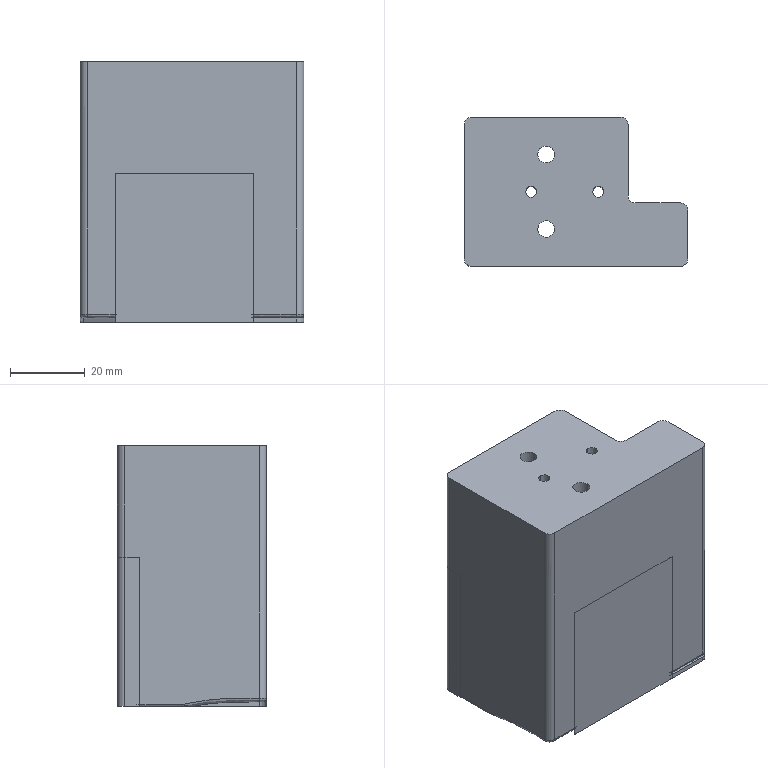NC program | NX | posted with a generic post | part box 60.004 x 40.015 x 70 mm
Lines 1 to 1318 of 2490:
N10 G17 G21 G94 G90
(FLOOR_WALL , TOOL : D63)
N12 T01 M6
N14 G54
N16 G17 G0 G90 X-72.5 Y32.997 B0. C0. S6500 M3
N18 G43 Z30. H1
N20 Z3.
N22 G94 G1 Z0. F1250.
N24 X-69.5
N26 X69.5
N28 Y12.597
N30 X-69.5
N32 Y-7.804
N34 X69.5
N36 X72.5
N38 Z3.
N40 G0 Z30.
N42 M5
(CAVITY_MILL , TOOL : D10)
N44 T09 M6
N46 G54
N48 G17 G0 G90 X4.33 Y-40. B0. C0. S9500 M3
N50 G43 Z30. H9
N52 Z0.504
N54 G94 G1 Z-0.996 F1000.
N56 X0.866 Y-34.
N58 G3 X0. Y-33.5 R1.
N60 G1 X-38.002 F3000.
N62 G2 X-38.495 Y-33.007 R0.493
N64 G1 Y-18.972
N66 G2 X-41.3 Y-13.732 R6.329
N68 G1 Y29.736
N70 G2 X-35. Y36.044 R6.328
N72 G1 X-5.019
N74 X35.006
N76 G2 X41.3 Y29.732 R6.327
N78 G1 Y-13.731
N80 G2 X38.495 Y-18.983 R6.306
N82 G1 Y-33.007
N84 G2 X38.002 Y-33.5 R0.493
N86 G1 X0.
N88 Y-27.5
N90 X-32.495
N92 Y-20.044
N94 X32.495
N96 Y-18.844
N98 X-35.
N100 G2 X-40.1 Y-13.732 R5.129
N102 G1 Y29.732
N104 G2 X-35. Y34.844 R5.128
N106 G1 X35.
N108 G2 X40.1 Y29.732 R5.127
N110 G1 Y-13.732
N112 G2 X35. Y-18.844 R5.106
N114 G1 X32.495
N116 Y-20.044
N118 Y-27.5
N120 X0.
N122 G3 X-0.866 Y-28. R1.
N124 G1 Y-40.
N126 Z0.504
N128 G0 X4.33 Z-0.491
N130 G1 Z-1.991 F1000.
N132 X0.866 Y-34.
N134 G3 X0. Y-33.5 R1.
N136 G1 X-38.002 F3000.
N138 G2 X-38.495 Y-33.007 R0.493
N140 G1 Y-19.24
N142 G2 X-41.3 Y-14. R6.299
N144 G1 Y30.
N146 G2 X-35. Y36.299 R6.3
N148 G1 X35.025 Y36.296
N150 X35.263 Y36.291
N152 G2 X41.3 Y30. R6.295
N154 G1 Y-14.
N156 G2 X38.495 Y-19.24 R6.3
N158 G1 Y-33.007
N160 G2 X38.002 Y-33.5 R0.493
N162 G1 X0.
N164 Y-27.5
N166 X-32.495
N168 Y-20.299
N170 X32.495
N172 Y-19.099
N174 X-35.001
N176 G2 X-40.1 Y-14. R5.099
N178 G1 Y30.
N180 G2 X-35. Y35.099 R5.1
N182 G1 X35. Y35.096
N184 X35.214 Y35.092
N186 G2 X40.1 Y30. R5.095
N188 G1 Y-14.
N190 G2 X35.013 Y-19.099 R5.1
N192 G1 X32.495
N194 Y-20.299
N196 Y-27.5
N198 X0.
N200 G3 X-0.866 Y-28. R1.
N202 G1 Y-40.
N204 Z-0.491
N206 G0 X4.33 Z-1.487
N208 G1 Z-2.987 F1000.
N210 X0.866 Y-34.
N212 G3 X0. Y-33.5 R1.
N214 G1 X-38.002 F3000.
N216 G2 X-38.496 Y-33.007 R0.493
N218 G1 Y-19.241
N220 G2 X-41.3 Y-14. R6.3
N222 G1 Y30.
N224 G2 X-35. Y36.3 R6.3
N226 G1 X35.
N228 G2 X41.3 Y30. R6.3
N230 G1 Y-14.
N232 G2 X38.496 Y-19.241 R6.3
N234 G1 Y-33.007
N236 G2 X38.002 Y-33.5 R0.493
N238 G1 X0.
N240 Y-27.5
N242 X-32.496
N244 Y-20.3
N246 X32.496
N248 Y-19.1
N250 X-35.
N252 G2 X-40.1 Y-14. R5.1
N254 G1 Y30.
N256 G2 X-35. Y35.1 R5.1
N258 G1 X35.
N260 G2 X40.1 Y30. R5.1
N262 G1 Y-14.
N264 G2 X35. Y-19.1 R5.1
N266 G1 X32.496
N268 Y-20.3
N270 Y-27.5
N272 X0.
N274 G3 X-0.866 Y-28. R1.
N276 G1 Y-40.
N278 Z-1.487
N280 G0 X4.33 Z-2.483
N282 G1 Z-3.983 F1000.
N284 X0.866 Y-34.
N286 G3 X0. Y-33.5 R1.
N288 G1 X-38.002 F3000.
N290 G2 X-38.496 Y-33.007 R0.493
N292 G1 Y-19.241
N294 G2 X-41.3 Y-14. R6.3
N296 G1 Y30.
N298 G2 X-35. Y36.3 R6.3
N300 G1 X35.
N302 G2 X41.3 Y30. R6.3
N304 G1 Y-14.
N306 G2 X38.496 Y-19.241 R6.3
N308 G1 Y-33.007
N310 G2 X38.002 Y-33.5 R0.493
N312 G1 X0.
N314 Y-27.5
N316 X-32.496
N318 Y-20.3
N320 X32.496
N322 Y-19.1
N324 X-35.
N326 G2 X-40.1 Y-14. R5.1
N328 G1 Y30.
N330 G2 X-35. Y35.1 R5.1
N332 G1 X35.
N334 G2 X40.1 Y30. R5.1
N336 G1 Y-14.
N338 G2 X35. Y-19.1 R5.1
N340 G1 X32.496
N342 Y-20.3
N344 Y-27.5
N346 X0.
N348 G3 X-0.866 Y-28. R1.
N350 G1 Y-40.
N352 Z-2.483
N354 G0 X4.33 Z-3.478
N356 G1 Z-4.978 F1000.
N358 X0.866 Y-34.
N360 G3 X0. Y-33.5 R1.
N362 G1 X-38.002 F3000.
N364 G2 X-38.496 Y-33.007 R0.494
N366 G1 Y-19.241
N368 G2 X-41.3 Y-14. R6.3
N370 G1 Y30.
N372 G2 X-35. Y36.3 R6.3
N374 G1 X35.
N376 G2 X41.3 Y30. R6.3
N378 G1 Y-14.
N380 G2 X38.496 Y-19.241 R6.3
N382 G1 Y-33.007
N384 G2 X38.002 Y-33.5 R0.494
N386 G1 X0.
N388 Y-27.5
N390 X-32.496
N392 Y-20.3
N394 X32.496
N396 Y-19.1
N398 X-35.
N400 G2 X-40.1 Y-14. R5.1
N402 G1 Y30.
N404 G2 X-35. Y35.1 R5.1
N406 G1 X35.
N408 G2 X40.1 Y30. R5.1
N410 G1 Y-14.
N412 G2 X35. Y-19.1 R5.1
N414 G1 X32.496
N416 Y-20.3
N418 Y-27.5
N420 X0.
N422 G3 X-0.866 Y-28. R1.
N424 G1 Y-40.
N426 Z-3.478
N428 G0 X4.33 Z-4.474
N430 G1 Z-5.974 F1000.
N432 X0.866 Y-34.
N434 G3 X0. Y-33.5 R1.
N436 G1 X-38.002 F3000.
N438 G2 X-38.496 Y-33.007 R0.494
N440 G1 Y-19.241
N442 G2 X-41.3 Y-14. R6.3
N444 G1 Y30.
N446 G2 X-35. Y36.3 R6.3
N448 G1 X35.
N450 G2 X41.3 Y30. R6.3
N452 G1 Y-14.
N454 G2 X38.496 Y-19.241 R6.3
N456 G1 Y-33.007
N458 G2 X38.002 Y-33.5 R0.494
N460 G1 X0.
N462 Y-27.5
N464 X-32.496
N466 Y-20.3
N468 X32.496
N470 Y-19.1
N472 X-35.
N474 G2 X-40.1 Y-14. R5.1
N476 G1 Y30.
N478 G2 X-35. Y35.1 R5.1
N480 G1 X35.
N482 G2 X40.1 Y30. R5.1
N484 G1 Y-14.
N486 G2 X35. Y-19.1 R5.1
N488 G1 X32.496
N490 Y-20.3
N492 Y-27.5
N494 X0.
N496 G3 X-0.866 Y-28. R1.
N498 G1 Y-40.
N500 Z-4.474
N502 G0 X4.33 Y-40.001 Z-5.47
N504 G1 Z-6.97 F1000.
N506 X0.866 Y-34.001
N508 G3 X0. Y-33.501 R1.
N510 G1 X-38.002 F3000.
N512 G2 X-38.496 Y-33.007 R0.494
N514 G1 Y-19.241
N516 G2 X-41.3 Y-14. R6.3
N518 G1 Y30.
N520 G2 X-35. Y36.3 R6.3
N522 G1 X35.
N524 G2 X41.3 Y30. R6.3
N526 G1 Y-14.
N528 G2 X38.496 Y-19.241 R6.3
N530 G1 Y-33.007
N532 G2 X38.002 Y-33.501 R0.494
N534 G1 X0.
N536 Y-27.501
N538 X-32.496
N540 Y-20.3
N542 X32.496
N544 Y-19.1
N546 X-35.
N548 G2 X-40.1 Y-14. R5.1
N550 G1 Y30.
N552 G2 X-35. Y35.1 R5.1
N554 G1 X35.
N556 G2 X40.1 Y30. R5.1
N558 G1 Y-14.
N560 G2 X35. Y-19.1 R5.1
N562 G1 X32.496
N564 Y-20.3
N566 Y-27.501
N568 X0.
N570 G3 X-0.866 Y-28.001 R1.
N572 G1 Y-40.001
N574 Z-5.47
N576 G0 X4.33 Z-6.465
N578 G1 Z-7.965 F1000.
N580 X0.866 Y-34.001
N582 G3 X0. Y-33.501 R1.
N584 G1 X-38.002 F3000.
N586 G2 X-38.496 Y-33.007 R0.494
N588 G1 Y-19.241
N590 G2 X-41.3 Y-14. R6.3
N592 G1 Y30.
N594 G2 X-35. Y36.3 R6.3
N596 G1 X35.
N598 G2 X41.3 Y30. R6.3
N600 G1 Y-14.
N602 G2 X38.496 Y-19.241 R6.3
N604 G1 Y-33.007
N606 G2 X38.002 Y-33.501 R0.494
N608 G1 X0.
N610 Y-27.501
N612 X-32.496
N614 Y-20.3
N616 X32.496
N618 Y-19.1
N620 X-35.
N622 G2 X-40.1 Y-14. R5.1
N624 G1 Y30.
N626 G2 X-35. Y35.1 R5.1
N628 G1 X35.
N630 G2 X40.1 Y30. R5.1
N632 G1 Y-14.
N634 G2 X35. Y-19.1 R5.1
N636 G1 X32.496
N638 Y-20.3
N640 Y-27.501
N642 X0.
N644 G3 X-0.866 Y-28.001 R1.
N646 G1 Y-40.001
N648 Z-6.465
N650 G0 X4.33 Z-7.461
N652 G1 Z-8.961 F1000.
N654 X0.866 Y-34.001
N656 G3 X0. Y-33.501 R1.
N658 G1 X-38.002 F3000.
N660 G2 X-38.496 Y-33.007 R0.494
N662 G1 Y-19.241
N664 G2 X-41.3 Y-14. R6.3
N666 G1 Y30.
N668 G2 X-35. Y36.3 R6.3
N670 G1 X35.
N672 G2 X41.3 Y30. R6.3
N674 G1 Y-14.
N676 G2 X38.496 Y-19.241 R6.3
N678 G1 Y-33.007
N680 G2 X38.002 Y-33.501 R0.494
N682 G1 X0.
N684 Y-27.501
N686 X-32.496
N688 Y-20.3
N690 X32.496
N692 Y-19.1
N694 X-35.
N696 G2 X-40.1 Y-14. R5.1
N698 G1 Y30.
N700 G2 X-35. Y35.1 R5.1
N702 G1 X35.
N704 G2 X40.1 Y30. R5.1
N706 G1 Y-14.
N708 G2 X35. Y-19.1 R5.1
N710 G1 X32.496
N712 Y-20.3
N714 Y-27.501
N716 X0.
N718 G3 X-0.866 Y-28.001 R1.
N720 G1 Y-40.001
N722 Z-7.461
N724 G0 X4.33 Z-8.457
N726 G1 Z-9.957 F1000.
N728 X0.866 Y-34.001
N730 G3 X0. Y-33.501 R1.
N732 G1 X-38.002 F3000.
N734 G2 X-38.496 Y-33.007 R0.494
N736 G1 Y-19.241
N738 G2 X-41.3 Y-14. R6.3
N740 G1 Y30.
N742 G2 X-35. Y36.3 R6.3
N744 G1 X35.
N746 G2 X41.3 Y30. R6.3
N748 G1 Y-14.
N750 G2 X38.496 Y-19.241 R6.3
N752 G1 Y-33.007
N754 G2 X38.002 Y-33.501 R0.494
N756 G1 X0.
N758 Y-27.501
N760 X-32.496
N762 Y-20.3
N764 X32.496
N766 Y-19.1
N768 X-35.
N770 G2 X-40.1 Y-14. R5.1
N772 G1 Y30.
N774 G2 X-35. Y35.1 R5.1
N776 G1 X35.
N778 G2 X40.1 Y30. R5.1
N780 G1 Y-14.
N782 G2 X35. Y-19.1 R5.1
N784 G1 X32.496
N786 Y-20.3
N788 Y-27.501
N790 X0.
N792 G3 X-0.866 Y-28.001 R1.
N794 G1 Y-40.001
N796 Z-8.457
N798 G0 X4.33 Z-9.452
N800 G1 Z-10.952 F1000.
N802 X0.866 Y-34.001
N804 G3 X0. Y-33.501 R1.
N806 G1 X-38.002 F3000.
N808 G2 X-38.496 Y-33.006 R0.494
N810 G1 Y-19.241
N812 G2 X-41.3 Y-14. R6.3
N814 G1 Y30.
N816 G2 X-35. Y36.3 R6.3
N818 G1 X35.
N820 G2 X41.3 Y30. R6.3
N822 G1 Y-14.
N824 G2 X38.496 Y-19.241 R6.3
N826 G1 Y-33.006
N828 G2 X38.002 Y-33.501 R0.494
N830 G1 X0.
N832 Y-27.501
N834 X-32.496
N836 Y-20.3
N838 X32.496
N840 Y-19.1
N842 X-35.
N844 G2 X-40.1 Y-14. R5.1
N846 G1 Y30.
N848 G2 X-35. Y35.1 R5.1
N850 G1 X35.
N852 G2 X40.1 Y30. R5.1
N854 G1 Y-14.
N856 G2 X35. Y-19.1 R5.1
N858 G1 X32.496
N860 Y-20.3
N862 Y-27.501
N864 X0.
N866 G3 X-0.866 Y-28.001 R1.
N868 G1 Y-40.001
N870 Z-9.452
N872 G0 X4.33 Z-10.448
N874 G1 Z-11.948 F1000.
N876 X0.866 Y-34.001
N878 G3 X0. Y-33.501 R1.
N880 G1 X-38.002 F3000.
N882 G2 X-38.497 Y-33.006 R0.495
N884 G1 Y-19.241
N886 G2 X-41.3 Y-14. R6.3
N888 G1 Y30.
N890 G2 X-35. Y36.3 R6.3
N892 G1 X35.
N894 G2 X41.3 Y30. R6.3
N896 G1 Y-14.
N898 G2 X38.497 Y-19.241 R6.3
N900 G1 Y-33.006
N902 G2 X38.002 Y-33.501 R0.495
N904 G1 X0.
N906 Y-27.501
N908 X-32.497
N910 Y-20.3
N912 X32.497
N914 Y-19.1
N916 X-35.
N918 G2 X-40.1 Y-14. R5.1
N920 G1 Y30.
N922 G2 X-35. Y35.1 R5.1
N924 G1 X35.
N926 G2 X40.1 Y30. R5.1
N928 G1 Y-14.
N930 G2 X35. Y-19.1 R5.1
N932 G1 X32.497
N934 Y-20.3
N936 Y-27.501
N938 X0.
N940 G3 X-0.866 Y-28.001 R1.
N942 G1 Y-40.001
N944 Z-10.448
N946 G0 X4.33 Z-11.443
N948 G1 Z-12.943 F1000.
N950 X0.866 Y-34.001
N952 G3 X0. Y-33.501 R1.
N954 G1 X-38.002 F3000.
N956 G2 X-38.497 Y-33.006 R0.495
N958 G1 Y-19.241
N960 G2 X-41.3 Y-14. R6.3
N962 G1 Y30.
N964 G2 X-35. Y36.3 R6.3
N966 G1 X35.
N968 G2 X41.3 Y30. R6.3
N970 G1 Y-14.
N972 G2 X38.497 Y-19.241 R6.3
N974 G1 Y-33.006
N976 G2 X38.002 Y-33.501 R0.495
N978 G1 X0.
N980 Y-27.501
N982 X-32.497
N984 Y-20.3
N986 X32.497
N988 Y-19.1
N990 X-35.
N992 G2 X-40.1 Y-14. R5.1
N994 G1 Y30.
N996 G2 X-35. Y35.1 R5.1
N998 G1 X35.
N1000 G2 X40.1 Y30. R5.1
N1002 G1 Y-14.
N1004 G2 X35. Y-19.1 R5.1
N1006 G1 X32.497
N1008 Y-20.3
N1010 Y-27.501
N1012 X0.
N1014 G3 X-0.866 Y-28.001 R1.
N1016 G1 Y-40.001
N1018 Z-11.443
N1020 G0 X4.33 Z-12.439
N1022 G1 Z-13.939 F1000.
N1024 X0.866 Y-34.001
N1026 G3 X0. Y-33.501 R1.
N1028 G1 X-38.002 F3000.
N1030 G2 X-38.497 Y-33.006 R0.495
N1032 G1 Y-19.24
N1034 G2 X-41.3 Y-14. R6.3
N1036 G1 Y30.
N1038 G2 X-35. Y36.3 R6.3
N1040 G1 X35.
N1042 G2 X41.3 Y30. R6.3
N1044 G1 Y-14.
N1046 G2 X38.497 Y-19.24 R6.3
N1048 G1 Y-33.006
N1050 G2 X38.002 Y-33.501 R0.495
N1052 G1 X0.
N1054 Y-27.501
N1056 X-32.497
N1058 Y-20.3
N1060 X32.497
N1062 Y-19.1
N1064 X-35.
N1066 G2 X-40.1 Y-14. R5.1
N1068 G1 Y30.
N1070 G2 X-35. Y35.1 R5.1
N1072 G1 X35.
N1074 G2 X40.1 Y30. R5.1
N1076 G1 Y-14.
N1078 G2 X35. Y-19.1 R5.1
N1080 G1 X32.497
N1082 Y-20.3
N1084 Y-27.501
N1086 X0.
N1088 G3 X-0.866 Y-28.001 R1.
N1090 G1 Y-40.001
N1092 Z-12.439
N1094 G0 X4.33 Z-13.435
N1096 G1 Z-14.935 F1000.
N1098 X0.866 Y-34.001
N1100 G3 X0. Y-33.501 R1.
N1102 G1 X-38.002 F3000.
N1104 G2 X-38.497 Y-33.006 R0.495
N1106 G1 Y-19.24
N1108 G2 X-41.3 Y-14. R6.3
N1110 G1 Y30.
N1112 G2 X-35. Y36.3 R6.3
N1114 G1 X35.
N1116 G2 X41.3 Y30. R6.3
N1118 G1 Y-14.
N1120 G2 X38.497 Y-19.24 R6.3
N1122 G1 Y-33.006
N1124 G2 X38.002 Y-33.501 R0.495
N1126 G1 X0.
N1128 Y-27.501
N1130 X-32.497
N1132 Y-20.3
N1134 X32.497
N1136 Y-19.1
N1138 X-35.
N1140 G2 X-40.1 Y-14. R5.1
N1142 G1 Y30.
N1144 G2 X-35. Y35.1 R5.1
N1146 G1 X35.
N1148 G2 X40.1 Y30. R5.1
N1150 G1 Y-14.
N1152 G2 X35. Y-19.1 R5.1
N1154 G1 X32.497
N1156 Y-20.3
N1158 Y-27.501
N1160 X0.
N1162 G3 X-0.866 Y-28.001 R1.
N1164 G1 Y-40.001
N1166 Z-13.435
N1168 G0 X4.33 Z-14.43
N1170 G1 Z-15.93 F1000.
N1172 X0.866 Y-34.001
N1174 G3 X0. Y-33.501 R1.
N1176 G1 X-38.002 F3000.
N1178 G2 X-38.497 Y-33.006 R0.495
N1180 G1 Y-19.24
N1182 G2 X-41.3 Y-14. R6.3
N1184 G1 Y30.
N1186 G2 X-35. Y36.3 R6.3
N1188 G1 X35.
N1190 G2 X41.3 Y30. R6.3
N1192 G1 Y-14.
N1194 G2 X38.497 Y-19.24 R6.3
N1196 G1 Y-33.006
N1198 G2 X38.002 Y-33.501 R0.495
N1200 G1 X0.
N1202 Y-27.501
N1204 X-32.497
N1206 Y-20.3
N1208 X32.497
N1210 Y-19.1
N1212 X-35.
N1214 G2 X-40.1 Y-14. R5.1
N1216 G1 Y30.
N1218 G2 X-35. Y35.1 R5.1
N1220 G1 X35.
N1222 G2 X40.1 Y30. R5.1
N1224 G1 Y-14.
N1226 G2 X35. Y-19.1 R5.1
N1228 G1 X32.497
N1230 Y-20.3
N1232 Y-27.501
N1234 X0.
N1236 G3 X-0.866 Y-28.001 R1.
N1238 G1 Y-40.001
N1240 Z-14.43
N1242 G0 X4.33 Z-15.426
N1244 G1 Z-16.926 F1000.
N1246 X0.866 Y-34.001
N1248 G3 X0. Y-33.501 R1.
N1250 G1 X-38.002 F3000.
N1252 G2 X-38.497 Y-33.006 R0.495
N1254 G1 Y-19.24
N1256 G2 X-41.3 Y-14. R6.3
N1258 G1 Y30.
N1260 G2 X-35. Y36.3 R6.3
N1262 G1 X35.
N1264 G2 X41.3 Y30. R6.3
N1266 G1 Y-14.
N1268 G2 X38.497 Y-19.24 R6.3
N1270 G1 Y-33.006
N1272 G2 X38.002 Y-33.501 R0.495
N1274 G1 X0.
N1276 Y-27.501
N1278 X-32.497
N1280 Y-20.3
N1282 X32.497
N1284 Y-19.1
N1286 X-35.
N1288 G2 X-40.1 Y-14. R5.1
N1290 G1 Y30.
N1292 G2 X-35. Y35.1 R5.1
N1294 G1 X35.
N1296 G2 X40.1 Y30. R5.1
N1298 G1 Y-14.
N1300 G2 X35. Y-19.1 R5.1
N1302 G1 X32.497
N1304 Y-20.3
N1306 Y-27.501
N1308 X0.
N1310 G3 X-0.866 Y-28.001 R1.
N1312 G1 Y-40.001
N1314 Z-15.426
N1316 G0 X4.33 Y-40.002 Z-16.422
N1318 G1 Z-17.922 F1000.
N1320 X0.866 Y-34.002
N1322 G3 X0. Y-33.502 R1.
N1324 G1 X-38.002 F3000.
N1326 G2 X-38.497 Y-33.006 R0.496
N1328 G1 Y-19.24
N1330 G2 X-41.3 Y-14. R6.3
N1332 G1 Y30.
N1334 G2 X-35. Y36.3 R6.3
N1336 G1 X35.
N1338 G2 X41.3 Y30. R6.3
N1340 G1 Y-14.
N1342 G2 X38.497 Y-19.24 R6.3
N1344 G1 Y-33.006
N1346 G2 X38.002 Y-33.502 R0.496
N1348 G1 X0.
N1350 Y-27.502
N1352 X-32.497
N1354 Y-20.3
N1356 X32.497
N1358 Y-19.1
N1360 X-35.
N1362 G2 X-40.1 Y-14. R5.1
N1364 G1 Y30.
N1366 G2 X-35. Y35.1 R5.1
N1368 G1 X35.
N1370 G2 X40.1 Y30. R5.1
N1372 G1 Y-14.
N1374 G2 X35. Y-19.1 R5.1
N1376 G1 X32.497
N1378 Y-20.3
N1380 Y-27.502
N1382 X0.
N1384 G3 X-0.866 Y-28.002 R1.
N1386 G1 Y-40.002
N1388 Z-16.422
N1390 G0 X4.33 Z-17.417
N1392 G1 Z-18.917 F1000.
N1394 X0.866 Y-34.002
N1396 G3 X0. Y-33.502 R1.
N1398 G1 X-38.002 F3000.
N1400 G2 X-38.497 Y-33.006 R0.496
N1402 G1 Y-19.24
N1404 G2 X-41.3 Y-14. R6.3
N1406 G1 Y30.
N1408 G2 X-35. Y36.3 R6.3
N1410 G1 X35.
N1412 G2 X41.3 Y30. R6.3
N1414 G1 Y-14.
N1416 G2 X38.497 Y-19.24 R6.3
N1418 G1 Y-33.006
N1420 G2 X38.002 Y-33.502 R0.496
N1422 G1 X0.
N1424 Y-27.502
N1426 X-32.497
N1428 Y-20.3
N1430 X32.497
N1432 Y-19.1
N1434 X-35.
N1436 G2 X-40.1 Y-14. R5.1
N1438 G1 Y30.
N1440 G2 X-35. Y35.1 R5.1
N1442 G1 X35.
N1444 G2 X40.1 Y30. R5.1
N1446 G1 Y-14.
N1448 G2 X35. Y-19.1 R5.1
N1450 G1 X32.497
N1452 Y-20.3
N1454 Y-27.502
N1456 X0.
N1458 G3 X-0.866 Y-28.002 R1.
N1460 G1 Y-40.002
N1462 Z-17.417
N1464 G0 X4.33 Z-18.413
N1466 G1 Z-19.913 F1000.
N1468 X0.866 Y-34.002
N1470 G3 X0. Y-33.502 R1.
N1472 G1 X-38.002 F3000.
N1474 G2 X-38.497 Y-33.006 R0.496
N1476 G1 Y-19.24
N1478 G2 X-41.3 Y-14. R6.3
N1480 G1 Y30.
N1482 G2 X-35. Y36.3 R6.3
N1484 G1 X35.
N1486 G2 X41.3 Y30. R6.3
N1488 G1 Y-14.
N1490 G2 X38.497 Y-19.24 R6.3
N1492 G1 Y-33.006
N1494 G2 X38.002 Y-33.502 R0.496
N1496 G1 X0.
N1498 Y-27.502
N1500 X-32.497
N1502 Y-20.3
N1504 X32.497
N1506 Y-19.1
N1508 X-35.
N1510 G2 X-40.1 Y-14. R5.1
N1512 G1 Y30.
N1514 G2 X-35. Y35.1 R5.1
N1516 G1 X35.
N1518 G2 X40.1 Y30. R5.1
N1520 G1 Y-14.
N1522 G2 X35. Y-19.1 R5.1
N1524 G1 X32.497
N1526 Y-20.3
N1528 Y-27.502
N1530 X0.
N1532 G3 X-0.866 Y-28.002 R1.
N1534 G1 Y-40.002
N1536 Z-18.413
N1538 G0 X4.33 Z-19.409
N1540 G1 Z-20.909 F1000.
N1542 X0.866 Y-34.002
N1544 G3 X0. Y-33.502 R1.
N1546 G1 X-38.001 F3000.
N1548 G2 X-38.497 Y-33.006 R0.496
N1550 G1 Y-19.24
N1552 G2 X-41.3 Y-14. R6.3
N1554 G1 Y30.
N1556 G2 X-35. Y36.3 R6.3
N1558 G1 X35.
N1560 G2 X41.3 Y30. R6.3
N1562 G1 Y-14.
N1564 G2 X38.497 Y-19.24 R6.3
N1566 G1 Y-33.006
N1568 G2 X38.001 Y-33.502 R0.496
N1570 G1 X0.
N1572 Y-27.502
N1574 X-32.497
N1576 Y-20.3
N1578 X32.497
N1580 Y-19.1
N1582 X-35.
N1584 G2 X-40.1 Y-14. R5.1
N1586 G1 Y30.
N1588 G2 X-35. Y35.1 R5.1
N1590 G1 X35.
N1592 G2 X40.1 Y30. R5.1
N1594 G1 Y-14.
N1596 G2 X35. Y-19.1 R5.1
N1598 G1 X32.497
N1600 Y-20.3
N1602 Y-27.502
N1604 X0.
N1606 G3 X-0.866 Y-28.002 R1.
N1608 G1 Y-40.002
N1610 Z-19.409
N1612 G0 X4.33 Z-20.404
N1614 G1 Z-21.904 F1000.
N1616 X0.866 Y-34.002
N1618 G3 X0. Y-33.502 R1.
N1620 G1 X-38.001 F3000.
N1622 G2 X-38.498 Y-33.006 R0.496
N1624 G1 Y-19.489
N1626 G2 X-41.3 Y-14.242 R6.275
N1628 G1 Y30.
N1630 G2 X-35. Y36.3 R6.3
N1632 G1 X35.
N1634 G2 X41.3 Y30. R6.3
N1636 G1 X41.299 Y-14.499
N1638 G2 X38.498 Y-19.498 R6.301
N1640 G1 Y-33.006
N1642 G2 X38.001 Y-33.502 R0.496
N1644 G1 X0.
N1646 Y-27.502
N1648 X-32.498
N1650 Y-20.529
N1652 X-5.469
N1654 X-5.127 Y-20.553
N1656 G3 X-4.485 Y-20.529 R3.949
N1658 G1 X32.498
N1660 Y-19.329
N1662 X-4.563
N1664 G2 X-5.043 Y-19.356 R2.749
N1666 G1 X-5.428 Y-19.329
N1668 X-34.933
N1670 X-35.276 Y-19.332
N1672 G2 X-36.667 Y-19.064 R3.572
N1674 X-40.1 Y-14.244 R5.075
N1676 G1 Y30.
N1678 G2 X-35. Y35.1 R5.1
N1680 G1 X35.
N1682 G2 X40.1 Y30. R5.1
N1684 G1 Y-14.452
N1686 G2 X35.982 Y-19.261 R5.101
N1688 G1 X35.214 Y-19.353
N1690 X34.931 Y-19.329
N1692 X32.498
N1694 Y-20.529
N1696 Y-27.502
N1698 X0.
N1700 G3 X-0.866 Y-28.002 R1.
N1702 G1 Y-40.002
N1704 Z-20.404
N1706 G0 X4.33 Z-21.4
N1708 G1 Z-22.9 F1000.
N1710 X0.866 Y-34.002
N1712 G3 X0. Y-33.502 R1.
N1714 G1 X-38.001 F3000.
N1716 G2 X-38.498 Y-33.006 R0.496
N1718 G1 Y-20.961
N1720 G2 X-41.281 Y-15.932 R6.373
N1722 G1 X-41.3 Y-15.363
N1724 Y30.
N1726 G2 X-35. Y36.3 R6.3
N1728 G1 X35.
N1730 G2 X41.3 Y30. R6.3
N1732 G1 Y-15.346
N1734 G2 X38.498 Y-20.999 R6.734
N1736 G1 Y-33.006
N1738 G2 X38.001 Y-33.502 R0.496
N1740 G1 X0.
N1742 Y-27.502
N1744 X-32.498
N1746 Y-22.031
N1748 X32.498
N1750 Y-20.831
N1752 X-35.5
N1754 G2 X-40.082 Y-15.89 R5.173
N1756 G1 X-40.1 Y-15.363
N1758 Y30.
N1760 G2 X-35. Y35.1 R5.1
N1762 G1 X35.
N1764 G2 X40.1 Y30. R5.1
N1766 G1 Y-15.363
N1768 G2 X36.621 Y-20.67 R5.534
N1770 G1 X35.02 Y-20.936
N1772 X35. Y-20.831
N1774 X32.498
N1776 Y-22.031
N1778 Y-27.502
N1780 X0.
N1782 G3 X-0.866 Y-28.002 R1.
N1784 G1 Y-40.002
N1786 Z-21.4
N1788 G0 X1.84 Y-36.758 Z-22.351
N1790 G1 Z-23.851 F1000.
N1792 X0.974 Y-35.258
N1794 G3 X0.108 Y-34.758 R1.
N1796 G1 X-35. F3000.
N1798 G2 X-40.1 Y-29.638 R5.11
N1800 G1 Y30.
N1802 G2 X-35. Y35.1 R5.1
N1804 G1 X35.
N1806 G2 X40.1 Y30. R5.1
N1808 G1 Y-29.583
N1810 G2 X35.214 Y-34.696 R5.142
N1812 G1 X34.445
N1814 G3 X33.071 Y-34.758 R11.921
N1816 G1 X0.108
N1818 G3 X-0.758 Y-35.258 R1.
N1820 G1 X-1.624 Y-36.758
N1822 Z-22.351
N1824 G0 X1.84 Y-37.091 Z-23.302
N1826 G1 Z-24.802 F1000.
N1828 X0.974 Y-35.591
N1830 G3 X0.108 Y-35.091 R1.
N1832 G1 X-35. F3000.
N1834 G2 X-40.1 Y-29.991 R5.1
N1836 G1 Y30.
N1838 G2 X-35. Y35.1 R5.1
N1840 G1 X35.
N1842 G2 X40.1 Y30. R5.1
N1844 G1 Y-29.985
N1846 G2 X35.214 Y-35.08 R5.127
N1848 G1 X33.292 Y-35.07
N1850 X33.042 Y-35.091
N1852 X0.108
N1854 G3 X-0.758 Y-35.591 R1.
N1856 G1 X-1.624 Y-37.091
N1858 Z-23.302
N1860 G0 X1.84 Y-37.1 Z-24.253
N1862 G1 Z-25.753 F1000.
N1864 X0.974 Y-35.6
N1866 G3 X0.108 Y-35.1 R1.
N1868 G1 X-35. F3000.
N1870 G2 X-40.1 Y-30. R5.1
N1872 G1 Y30.
N1874 G2 X-35. Y35.1 R5.1
N1876 G1 X35.
N1878 G2 X40.1 Y30. R5.1
N1880 G1 Y-30.014
N1882 G2 X35.02 Y-35.096 R5.081
N1884 G1 X33.038
N1886 X33.004 Y-35.1
N1888 X0.108
N1890 G3 X-0.758 Y-35.6 R1.
N1892 G1 X-1.624 Y-37.1
N1894 Z-24.253
N1896 G0 X1.84 Z-25.203
N1898 G1 Z-26.703 F1000.
N1900 X0.974 Y-35.6
N1902 G3 X0.108 Y-35.1 R1.
N1904 G1 X-35. F3000.
N1906 G2 X-40.1 Y-30. R5.1
N1908 G1 Y30.
N1910 G2 X-35. Y35.1 R5.1
N1912 G1 X35.
N1914 G2 X40.1 Y30. R5.1
N1916 G1 Y-30.015
N1918 G2 X35.021 Y-35.096 R5.081
N1920 G1 X33.038
N1922 X33.004 Y-35.1
N1924 X0.108
N1926 G3 X-0.758 Y-35.6 R1.
N1928 G1 X-1.624 Y-37.1
N1930 Z-25.203
N1932 G0 X1.84 Z-26.154
N1934 G1 Z-27.654 F1000.
N1936 X0.974 Y-35.6
N1938 G3 X0.108 Y-35.1 R1.
N1940 G1 X-35. F3000.
N1942 G2 X-40.1 Y-30. R5.1
N1944 G1 Y30.
N1946 G2 X-35. Y35.1 R5.1
N1948 G1 X35.
N1950 G2 X40.1 Y30. R5.1
N1952 G1 Y-30.015
N1954 G2 X35.021 Y-35.096 R5.081
N1956 G1 X33.038
N1958 X33.004 Y-35.1
N1960 X0.108
N1962 G3 X-0.758 Y-35.6 R1.
N1964 G1 X-1.624 Y-37.1
N1966 Z-26.154
N1968 G0 X1.84 Z-27.105
N1970 G1 Z-28.605 F1000.
N1972 X0.974 Y-35.6
N1974 G3 X0.108 Y-35.1 R1.
N1976 G1 X-35. F3000.
N1978 G2 X-40.1 Y-30. R5.1
N1980 G1 Y30.
N1982 G2 X-35. Y35.1 R5.1
N1984 G1 X35.
N1986 G2 X40.1 Y30. R5.1
N1988 G1 Y-30.015
N1990 G2 X35.021 Y-35.096 R5.081
N1992 G1 X33.038
N1994 X33.004 Y-35.1
N1996 X0.108
N1998 G3 X-0.758 Y-35.6 R1.
N2000 G1 X-1.624 Y-37.1
N2002 Z-27.105
N2004 G0 X1.84 Z-28.056
N2006 G1 Z-29.556 F1000.
N2008 X0.974 Y-35.6
N2010 G3 X0.108 Y-35.1 R1.
N2012 G1 X-35. F3000.
N2014 G2 X-40.1 Y-30. R5.1
N2016 G1 Y30.
N2018 G2 X-35. Y35.1 R5.1
N2020 G1 X35.
N2022 G2 X40.1 Y30. R5.1
N2024 G1 Y-30.016
N2026 G2 X35.021 Y-35.096 R5.08
N2028 G1 X33.038
N2030 X33.004 Y-35.1
N2032 X0.108
N2034 G3 X-0.758 Y-35.6 R1.
N2036 G1 X-1.624 Y-37.1
N2038 Z-28.056
N2040 G0 X1.84 Z-29.007
N2042 G1 Z-30.507 F1000.
N2044 X0.974 Y-35.6
N2046 G3 X0.108 Y-35.1 R1.
N2048 G1 X-35. F3000.
N2050 G2 X-40.1 Y-30. R5.1
N2052 G1 Y30.
N2054 G2 X-35. Y35.1 R5.1
N2056 G1 X35.
N2058 G2 X40.1 Y30. R5.1
N2060 G1 Y-30.016
N2062 G2 X35.021 Y-35.096 R5.08
N2064 G1 X33.038 Y-35.097
N2066 X33.004 Y-35.1
N2068 X0.108
N2070 G3 X-0.758 Y-35.6 R1.
N2072 G1 X-1.624 Y-37.1
N2074 Z-29.007
N2076 G0 X1.84 Z-29.958
N2078 G1 Z-31.458 F1000.
N2080 X0.974 Y-35.6
N2082 G3 X0.108 Y-35.1 R1.
N2084 G1 X-35. F3000.
N2086 G2 X-40.1 Y-30. R5.1
N2088 G1 Y30.
N2090 G2 X-35. Y35.1 R5.1
N2092 G1 X35.
N2094 G2 X40.1 Y30. R5.1
N2096 G1 Y-30.016
N2098 G2 X35.021 Y-35.096 R5.08
N2100 G1 X33.038 Y-35.097
N2102 X33.004 Y-35.1
N2104 X0.108
N2106 G3 X-0.758 Y-35.6 R1.
N2108 G1 X-1.624 Y-37.1
N2110 Z-29.958
N2112 G0 X1.84 Z-30.908
N2114 G1 Z-32.408 F1000.
N2116 X0.974 Y-35.6
N2118 G3 X0.108 Y-35.1 R1.
N2120 G1 X-35. F3000.
N2122 G2 X-40.1 Y-30. R5.1
N2124 G1 Y30.
N2126 G2 X-35. Y35.1 R5.1
N2128 G1 X35.
N2130 G2 X40.1 Y30. R5.1
N2132 G1 Y-30.016
N2134 G2 X35.022 Y-35.096 R5.08
N2136 G1 X33.038 Y-35.097
N2138 X33.004 Y-35.1
N2140 X0.108
N2142 G3 X-0.758 Y-35.6 R1.
N2144 G1 X-1.624 Y-37.1
N2146 Z-30.908
N2148 G0 X1.84 Z-31.859
N2150 G1 Z-33.359 F1000.
N2152 X0.974 Y-35.6
N2154 G3 X0.108 Y-35.1 R1.
N2156 G1 X-35. F3000.
N2158 G2 X-40.1 Y-30. R5.1
N2160 G1 Y30.
N2162 G2 X-35. Y35.1 R5.1
N2164 G1 X35.
N2166 G2 X40.1 Y30. R5.1
N2168 G1 Y-30.017
N2170 G2 X35.022 Y-35.096 R5.08
N2172 G1 X33.038 Y-35.097
N2174 X33.004 Y-35.1
N2176 X0.108
N2178 G3 X-0.758 Y-35.6 R1.
N2180 G1 X-1.624 Y-37.1
N2182 Z-31.859
N2184 G0 X1.84 Z-32.81
N2186 G1 Z-34.31 F1000.
N2188 X0.974 Y-35.6
N2190 G3 X0.108 Y-35.1 R1.
N2192 G1 X-35. F3000.
N2194 G2 X-40.1 Y-30. R5.1
N2196 G1 Y30.
N2198 G2 X-35. Y35.1 R5.1
N2200 G1 X35.
N2202 G2 X40.1 Y30. R5.1
N2204 G1 Y-30.017
N2206 G2 X35.022 Y-35.096 R5.079
N2208 G1 X33.038 Y-35.097
N2210 X33.004 Y-35.1
N2212 X0.108
N2214 G3 X-0.758 Y-35.6 R1.
N2216 G1 X-1.624 Y-37.1
N2218 Z-32.81
N2220 G0 X1.84 Z-33.761
N2222 G1 Z-35.261 F1000.
N2224 X0.974 Y-35.6
N2226 G3 X0.108 Y-35.1 R1.
N2228 G1 X-35. F3000.
N2230 G2 X-40.1 Y-30. R5.1
N2232 G1 Y30.
N2234 G2 X-35. Y35.1 R5.1
N2236 G1 X35.
N2238 G2 X40.1 Y30. R5.1
N2240 G1 Y-30.017
N2242 G2 X35.022 Y-35.096 R5.079
N2244 G1 X33.038 Y-35.097
N2246 X33.004 Y-35.1
N2248 X0.108
N2250 G3 X-0.758 Y-35.6 R1.
N2252 G1 X-1.624 Y-37.1
N2254 Z-33.761
N2256 G0 X1.84 Z-34.712
N2258 G1 Z-36.212 F1000.
N2260 X0.974 Y-35.6
N2262 G3 X0.108 Y-35.1 R1.
N2264 G1 X-35. F3000.
N2266 G2 X-40.1 Y-30. R5.1
N2268 G1 Y30.
N2270 G2 X-35. Y35.1 R5.1
N2272 G1 X35.
N2274 G2 X40.1 Y30. R5.1
N2276 G1 Y-30.017
N2278 G2 X35.022 Y-35.096 R5.079
N2280 G1 X33.038 Y-35.097
N2282 X33.004 Y-35.1
N2284 X0.108
N2286 G3 X-0.758 Y-35.6 R1.
N2288 G1 X-1.624 Y-37.1
N2290 Z-34.712
N2292 G0 X1.84 Z-35.663
N2294 G1 Z-37.163 F1000.
N2296 X0.974 Y-35.6
N2298 G3 X0.108 Y-35.1 R1.
N2300 G1 X-35. F3000.
N2302 G2 X-40.1 Y-30. R5.1
N2304 G1 Y30.
N2306 G2 X-35. Y35.1 R5.1
N2308 G1 X35.
N2310 G2 X40.1 Y30. R5.1
N2312 G1 Y-30.017
N2314 G2 X35.022 Y-35.096 R5.079
N2316 G1 X33.038 Y-35.097
N2318 X33.004 Y-35.1
N2320 X0.108
N2322 G3 X-0.758 Y-35.6 R1.
N2324 G1 X-1.624 Y-37.1
N2326 Z-35.663
N2328 G0 X1.84 Z-36.613
N2330 G1 Z-38.113 F1000.
N2332 X0.974 Y-35.6
N2334 G3 X0.108 Y-35.1 R1.
N2336 G1 X-35. F3000.
N2338 G2 X-40.1 Y-30. R5.1
N2340 G1 Y30.
N2342 G2 X-35. Y35.1 R5.1
N2344 G1 X35.
N2346 G2 X40.1 Y30. R5.1
N2348 G1 Y-30.005
N2350 G2 X35.009 Y-35.096 R5.092
N2352 G1 X33.038 Y-35.097
N2354 X33.004 Y-35.1
N2356 X0.108
N2358 G3 X-0.758 Y-35.6 R1.
N2360 G1 X-1.624 Y-37.1
N2362 Z-36.613
N2364 G0 X1.84 Z-37.564
N2366 G1 Z-39.064 F1000.
N2368 X0.974 Y-35.6
N2370 G3 X0.108 Y-35.1 R1.
N2372 G1 X-35. F3000.
N2374 G2 X-40.1 Y-30. R5.1
N2376 G1 Y30.
N2378 G2 X-35. Y35.1 R5.1
N2380 G1 X35.
N2382 G2 X40.1 Y30. R5.1
N2384 G1 Y-30.005
N2386 G2 X35.009 Y-35.096 R5.092
N2388 G1 X33.038 Y-35.097
N2390 X33.004 Y-35.1
N2392 X0.108
N2394 G3 X-0.758 Y-35.6 R1.
N2396 G1 X-1.624 Y-37.1
N2398 Z-37.564
N2400 G0 X1.84 Z-38.515
N2402 G1 Z-40.015 F1000.
N2404 X0.974 Y-35.6
N2406 G3 X0.108 Y-35.1 R1.
N2408 G1 X-35. F3000.
N2410 G2 X-40.1 Y-30. R5.1
N2412 G1 Y30.
N2414 G2 X-35. Y35.1 R5.1
N2416 G1 X35.
N2418 G2 X40.1 Y30. R5.1
N2420 G1 Y-30.005
N2422 G2 X35.009 Y-35.096 R5.092
N2424 G1 X33.038 Y-35.097
N2426 X33.004 Y-35.1
N2428 X0.108
N2430 G3 X-0.758 Y-35.6 R1.
N2432 G1 X-1.624 Y-37.1
N2434 Z-38.515
N2436 G0 Z30.
N2438 M5
(ZLEVEL_PROFILE_COPY_COPY , TOOL : D10JING)
N2440 T10 M6
N2442 G54
N2444 G17 G0 G90 X-36.622 Y36.809 B0. C0. S9500 M3
N2446 G43 Z30. H10
N2448 Z-18.5
N2450 G94 G1 Z-20. F1000.
N2452 X-35.866 Y35.5
N2454 G3 X-35. Y35. R1.
N2456 G1 X35. F1200.
N2458 G2 X40. Y30. R5.
N2460 G1 Y-29.998
N2462 G2 X34.998 Y-35.001 R5.
N2464 G1 X33.661 Y-34.997
N2466 X33.438 Y-34.985
N2468 G2 X33.032 Y-35. R27.448
N2470 G1 X-35.
N2472 G2 X-40. Y-30. R5.
N2474 G1 Y30.
N2476 G2 X-35. Y35. R5.
N2478 G3 X-34.134 Y35.5 R1.
N2480 G1 X-33.268 Y37.
N2482 Z-18.5
N2484 G0 Z30.
N2486 X-36.622 Y36.809
N2488 Z-38.5
N2490 G1 Z-40. F1000.
N2492 X-35.866 Y35.5
N2494 G3 X-35. Y35. R1.
N2496 G1 X35. F1200.
N2498 G2 X40. Y30. R5.
N2500 G1 Y-29.998
N2502 G2 X34.998 Y-35.001 R5.
N2504 G1 X33.661 Y-34.997
N2506 X33.438 Y-34.985
N2508 G2 X33.032 Y-35. R27.238
N2510 G1 X-35.
N2512 G2 X-40. Y-30. R5.
N2514 G1 Y30.
N2516 G2 X-35. Y35. R5.
N2518 G3 X-34.134 Y35.5 R1.
N2520 G1 X-33.268 Y37.
N2522 Z-38.5
N2524 G0 Z30.
(ZLEVEL_PROFILE_COPY_COPY_COPY , TOOL : D10JING)
N2526 X-36.622 Y36.809
N2528 Z-19.5
N2530 G1 Z-21. F1000.
N2532 X-35.866 Y35.5
N2534 G3 X-35. Y35. R1.
N2536 G1 X35. F1200.
N2538 G2 X40. Y30. R5.
N2540 G1 Y-14.
N2542 G2 X35. Y-19. R5.
N2544 G1 X-35.
N2546 G2 X-40. Y-14. R5.
N2548 G1 Y30.
N2550 G2 X-35. Y35. R5.
N2552 G3 X-34.134 Y35.5 R1.
N2554 G1 X-33.268 Y37.
N2556 Z-19.5
N2558 G0 Z30.
(FLOOR_WALL_1 , TOOL : D10JING)
N2560 X39.599 Y-29.584
N2562 Z-21.5
N2564 G1 Z-23. F1000.
N2566 X38.972 Y-28.497
N2568 G3 X38.106 Y-27.997 R1.
N2570 G1 X-40.
N2572 Y-24.749
N2574 X38.119
N2576 X40. Y-24.519
N2578 Y-21.5
N2580 X-40.
N2582 G3 X-40.866 Y-22. R1.
N2584 G1 X-41.5 Y-23.098
N2586 Z-21.5
N2588 G0 Z30.
N2590 X41.5 Y-22.598
N2592 Z-21.5
N2594 G1 Z-23.
N2596 X40.866 Y-21.5
N2598 G3 X40. Y-21. R1.
N2600 G1 X-40.
N2602 G3 X-40.866 Y-21.5 R1.
N2604 G1 X-41.5 Y-22.598
N2606 Z-21.5
N2608 G0 Z30.
N2610 M5